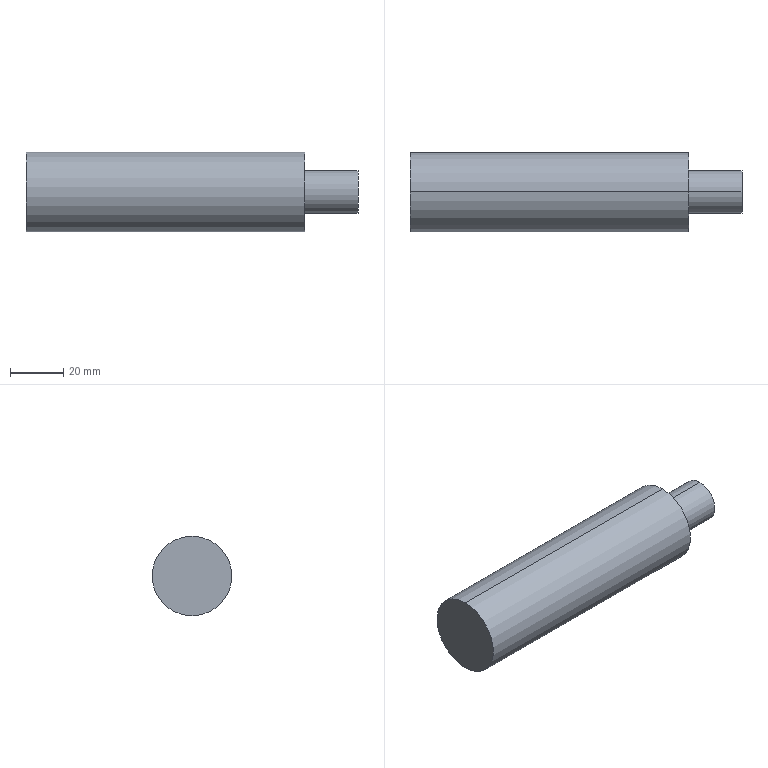Part | SolidWorks | features Revolution 1 | 1 solid | 7 faces | box 125 x 30 x 30 mm | volume 78241 mm3 | cylinder 4 | plane 3 | commonest cylinder face diameters 16 x2 30 x2
STEP:
#1=CARTESIAN_POINT('',(125.,0.,8.));
#2=VERTEX_POINT('',#1);
#3=CARTESIAN_POINT('',(125.,0.,-8.));
#4=VERTEX_POINT('',#3);
#5=CARTESIAN_POINT('',(125.,0.,0.));
#6=DIRECTION('',(-1.,0.,0.));
#7=DIRECTION('',(0.,0.,1.));
#8=AXIS2_PLACEMENT_3D('',#5,#6,#7);
#9=CIRCLE('',#8,8.);
#10=EDGE_CURVE('',#2,#4,#9,.T.);
#11=ORIENTED_EDGE('',*,*,#10,.T.);
#12=CARTESIAN_POINT('',(105.,0.,-8.));
#13=VERTEX_POINT('',#12);
#14=CARTESIAN_POINT('',(0.,0.,-8.));
#15=DIRECTION('',(-1.,0.,0.));
#16=VECTOR('',#15,1000.);
#17=LINE('',#14,#16);
#18=EDGE_CURVE('',#4,#13,#17,.T.);
#19=ORIENTED_EDGE('',*,*,#18,.T.);
#20=CARTESIAN_POINT('',(105.,0.,8.));
#21=VERTEX_POINT('',#20);
#22=CARTESIAN_POINT('',(105.,0.,0.));
#23=DIRECTION('',(-1.,0.,0.));
#24=DIRECTION('',(0.,0.,1.));
#25=AXIS2_PLACEMENT_3D('',#22,#23,#24);
#26=CIRCLE('',#25,8.);
#27=EDGE_CURVE('',#21,#13,#26,.T.);
#28=ORIENTED_EDGE('',*,*,#27,.F.);
#29=CARTESIAN_POINT('',(0.,0.,8.));
#30=DIRECTION('',(-1.,0.,0.));
#31=VECTOR('',#30,1000.);
#32=LINE('',#29,#31);
#33=EDGE_CURVE('',#2,#21,#32,.T.);
#34=ORIENTED_EDGE('',*,*,#33,.F.);
#35=EDGE_LOOP('',(#11,#19,#28,#34));
#36=FACE_OUTER_BOUND('',#35,.T.);
#37=CARTESIAN_POINT('',(0.,0.,0.));
#38=DIRECTION('',(-1.,0.,0.));
#39=DIRECTION('',(0.,0.,1.));
#40=AXIS2_PLACEMENT_3D('',#37,#38,#39);
#41=CYLINDRICAL_SURFACE('',#40,8.);
#42=ADVANCED_FACE('',(#36),#41,.T.);
#43=CARTESIAN_POINT('',(105.,0.,15.));
#44=VERTEX_POINT('',#43);
#45=CARTESIAN_POINT('',(105.,0.,-15.));
#46=VERTEX_POINT('',#45);
#47=CARTESIAN_POINT('',(105.,0.,0.));
#48=DIRECTION('',(-1.,0.,0.));
#49=DIRECTION('',(0.,0.,1.));
#50=AXIS2_PLACEMENT_3D('',#47,#48,#49);
#51=CIRCLE('',#50,15.);
#52=EDGE_CURVE('',#44,#46,#51,.T.);
#53=ORIENTED_EDGE('',*,*,#52,.T.);
#54=CARTESIAN_POINT('',(0.,0.,-15.));
#55=VERTEX_POINT('',#54);
#56=CARTESIAN_POINT('',(0.,0.,-15.));
#57=DIRECTION('',(-1.,0.,0.));
#58=VECTOR('',#57,1000.);
#59=LINE('',#56,#58);
#60=EDGE_CURVE('',#46,#55,#59,.T.);
#61=ORIENTED_EDGE('',*,*,#60,.T.);
#62=CARTESIAN_POINT('',(0.,0.,15.));
#63=VERTEX_POINT('',#62);
#64=CARTESIAN_POINT('',(0.,0.,0.));
#65=DIRECTION('',(-1.,0.,0.));
#66=DIRECTION('',(0.,0.,1.));
#67=AXIS2_PLACEMENT_3D('',#64,#65,#66);
#68=CIRCLE('',#67,15.);
#69=EDGE_CURVE('',#63,#55,#68,.T.);
#70=ORIENTED_EDGE('',*,*,#69,.F.);
#71=CARTESIAN_POINT('',(0.,0.,15.));
#72=DIRECTION('',(-1.,0.,0.));
#73=VECTOR('',#72,1000.);
#74=LINE('',#71,#73);
#75=EDGE_CURVE('',#44,#63,#74,.T.);
#76=ORIENTED_EDGE('',*,*,#75,.F.);
#77=EDGE_LOOP('',(#53,#61,#70,#76));
#78=FACE_OUTER_BOUND('',#77,.T.);
#79=CARTESIAN_POINT('',(0.,0.,0.));
#80=DIRECTION('',(-1.,0.,0.));
#81=DIRECTION('',(0.,0.,1.));
#82=AXIS2_PLACEMENT_3D('',#79,#80,#81);
#83=CYLINDRICAL_SURFACE('',#82,15.);
#84=ADVANCED_FACE('',(#78),#83,.T.);
#85=ORIENTED_EDGE('',*,*,#69,.T.);
#86=CARTESIAN_POINT('',(0.,0.,0.));
#87=DIRECTION('',(-1.,0.,0.));
#88=DIRECTION('',(0.,0.,1.));
#89=AXIS2_PLACEMENT_3D('',#86,#87,#88);
#90=CIRCLE('',#89,15.);
#91=EDGE_CURVE('',#55,#63,#90,.T.);
#92=ORIENTED_EDGE('',*,*,#91,.T.);
#93=EDGE_LOOP('',(#85,#92));
#94=FACE_OUTER_BOUND('',#93,.T.);
#95=CARTESIAN_POINT('',(0.,0.,0.));
#96=DIRECTION('',(1.,0.,0.));
#97=DIRECTION('',(0.,0.,-1.));
#98=AXIS2_PLACEMENT_3D('',#95,#96,#97);
#99=PLANE('',#98);
#100=ADVANCED_FACE('',(#94),#99,.F.);
#101=ORIENTED_EDGE('',*,*,#60,.F.);
#102=CARTESIAN_POINT('',(105.,0.,0.));
#103=DIRECTION('',(-1.,0.,0.));
#104=DIRECTION('',(0.,0.,1.));
#105=AXIS2_PLACEMENT_3D('',#102,#103,#104);
#106=CIRCLE('',#105,15.);
#107=EDGE_CURVE('',#46,#44,#106,.T.);
#108=ORIENTED_EDGE('',*,*,#107,.T.);
#109=ORIENTED_EDGE('',*,*,#75,.T.);
#110=ORIENTED_EDGE('',*,*,#91,.F.);
#111=EDGE_LOOP('',(#101,#108,#109,#110));
#112=FACE_OUTER_BOUND('',#111,.T.);
#113=CARTESIAN_POINT('',(0.,0.,0.));
#114=DIRECTION('',(-1.,0.,0.));
#115=DIRECTION('',(0.,0.,1.));
#116=AXIS2_PLACEMENT_3D('',#113,#114,#115);
#117=CYLINDRICAL_SURFACE('',#116,15.);
#118=ADVANCED_FACE('',(#112),#117,.T.);
#119=ORIENTED_EDGE('',*,*,#52,.F.);
#120=ORIENTED_EDGE('',*,*,#107,.F.);
#121=EDGE_LOOP('',(#119,#120));
#122=FACE_OUTER_BOUND('',#121,.T.);
#123=ORIENTED_EDGE('',*,*,#27,.T.);
#124=CARTESIAN_POINT('',(105.,0.,0.));
#125=DIRECTION('',(-1.,0.,0.));
#126=DIRECTION('',(0.,0.,1.));
#127=AXIS2_PLACEMENT_3D('',#124,#125,#126);
#128=CIRCLE('',#127,8.);
#129=EDGE_CURVE('',#13,#21,#128,.T.);
#130=ORIENTED_EDGE('',*,*,#129,.T.);
#131=EDGE_LOOP('',(#123,#130));
#132=FACE_BOUND('',#131,.T.);
#133=CARTESIAN_POINT('',(105.,15.,0.));
#134=DIRECTION('',(-1.,0.,0.));
#135=DIRECTION('',(0.,0.,1.));
#136=AXIS2_PLACEMENT_3D('',#133,#134,#135);
#137=PLANE('',#136);
#138=ADVANCED_FACE('',(#122,#132),#137,.F.);
#139=ORIENTED_EDGE('',*,*,#18,.F.);
#140=CARTESIAN_POINT('',(125.,0.,0.));
#141=DIRECTION('',(-1.,0.,0.));
#142=DIRECTION('',(0.,0.,1.));
#143=AXIS2_PLACEMENT_3D('',#140,#141,#142);
#144=CIRCLE('',#143,8.);
#145=EDGE_CURVE('',#4,#2,#144,.T.);
#146=ORIENTED_EDGE('',*,*,#145,.T.);
#147=ORIENTED_EDGE('',*,*,#33,.T.);
#148=ORIENTED_EDGE('',*,*,#129,.F.);
#149=EDGE_LOOP('',(#139,#146,#147,#148));
#150=FACE_OUTER_BOUND('',#149,.T.);
#151=CARTESIAN_POINT('',(0.,0.,0.));
#152=DIRECTION('',(-1.,0.,0.));
#153=DIRECTION('',(0.,0.,1.));
#154=AXIS2_PLACEMENT_3D('',#151,#152,#153);
#155=CYLINDRICAL_SURFACE('',#154,8.);
#156=ADVANCED_FACE('',(#150),#155,.T.);
#157=ORIENTED_EDGE('',*,*,#10,.F.);
#158=ORIENTED_EDGE('',*,*,#145,.F.);
#159=EDGE_LOOP('',(#157,#158));
#160=FACE_OUTER_BOUND('',#159,.T.);
#161=CARTESIAN_POINT('',(125.,8.,0.));
#162=DIRECTION('',(-1.,0.,0.));
#163=DIRECTION('',(0.,0.,1.));
#164=AXIS2_PLACEMENT_3D('',#161,#162,#163);
#165=PLANE('',#164);
#166=ADVANCED_FACE('',(#160),#165,.F.);
#167=CLOSED_SHELL('',(#42,#84,#100,#118,#138,#156,#166));
#168=MANIFOLD_SOLID_BREP('',#167);
#169=CARTESIAN_POINT('',(0.,0.,0.));
#170=DIRECTION('',(0.,0.,1.));
#171=DIRECTION('',(1.,0.,0.));
#172=AXIS2_PLACEMENT_3D('',#169,#170,#171);
#173=(LENGTH_UNIT()NAMED_UNIT(*)SI_UNIT(.MILLI.,.METRE.));
#174=UNCERTAINTY_MEASURE_WITH_UNIT(LENGTH_MEASURE(0.00001),#173,'','');
#175=(NAMED_UNIT(*)PLANE_ANGLE_UNIT()SI_UNIT($,.RADIAN.));
#176=(NAMED_UNIT(*)SI_UNIT($,.STERADIAN.)SOLID_ANGLE_UNIT());
#177=(GEOMETRIC_REPRESENTATION_CONTEXT(3)GLOBAL_UNCERTAINTY_ASSIGNED_CONTEXT((#174))GLOBAL_UNIT_ASSIGNED_CONTEXT((#173,#175,#176))REPRESENTATION_CONTEXT('',''));
#178=ADVANCED_BREP_SHAPE_REPRESENTATION('',(#168,#172),#177);